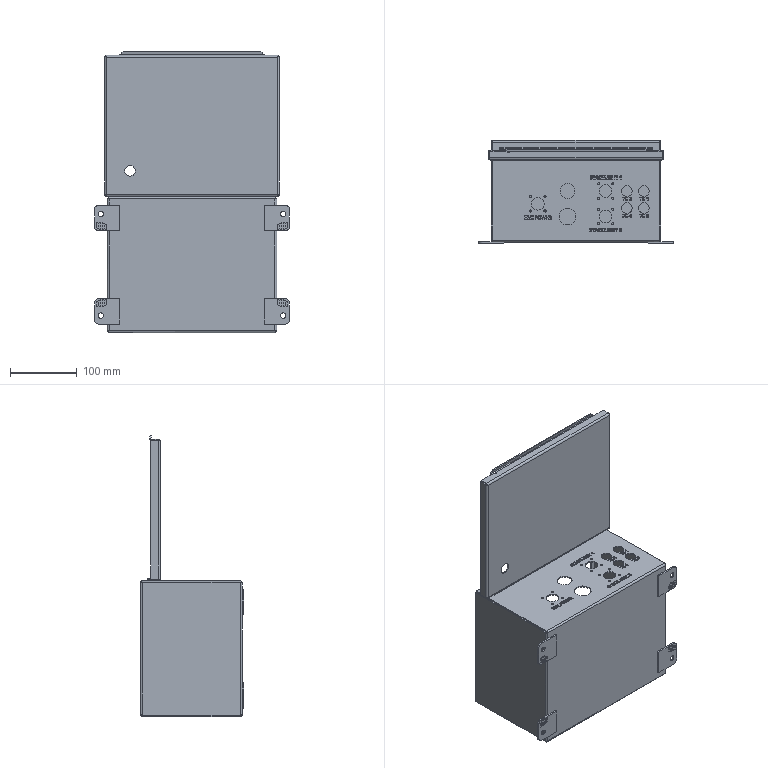Part | SolidWorks | 4 solids | 1349 faces | box 292.1 x 154.813 x 421.143 mm | volume 614239 mm3 | plane 712 | cylinder 390 | spline 211 | cone 32 | torus 4 | commonest cylinder face diameters 2.54 x36 12.7 x29 3.175 x24 1.27 x18 1.829 x15 5.486 x14